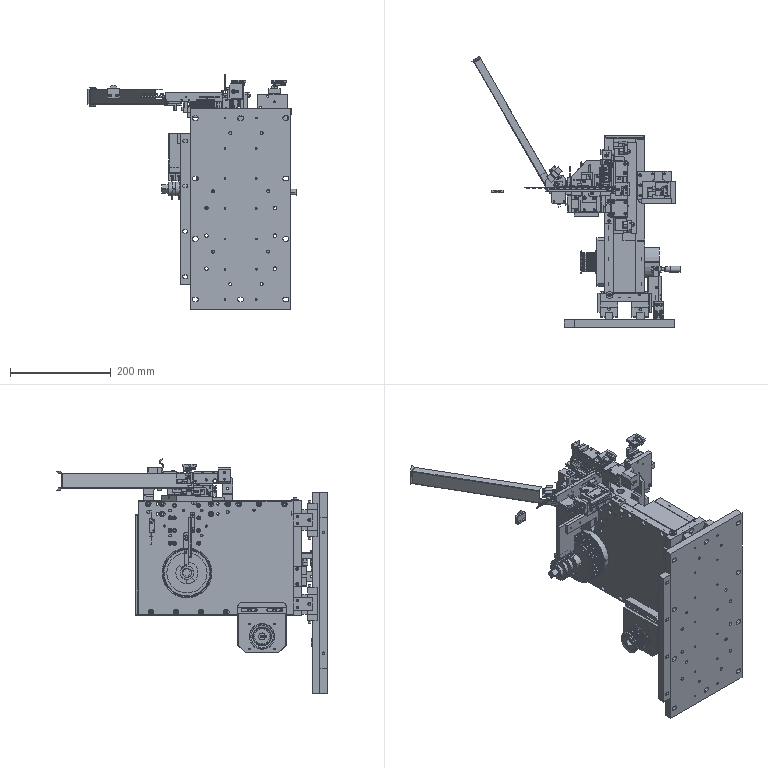Part | NX | 214 solids | 14997 faces | volume 6657235 mm3 | plane 7938 | cylinder 4982 | cone 1433 | torus 357 | spline 183 | sphere 104 | commonest cylinder face diameters 5 x559 0.3 x320 0.2 x316 3.3 x290 0.5 x280 2.5 x191